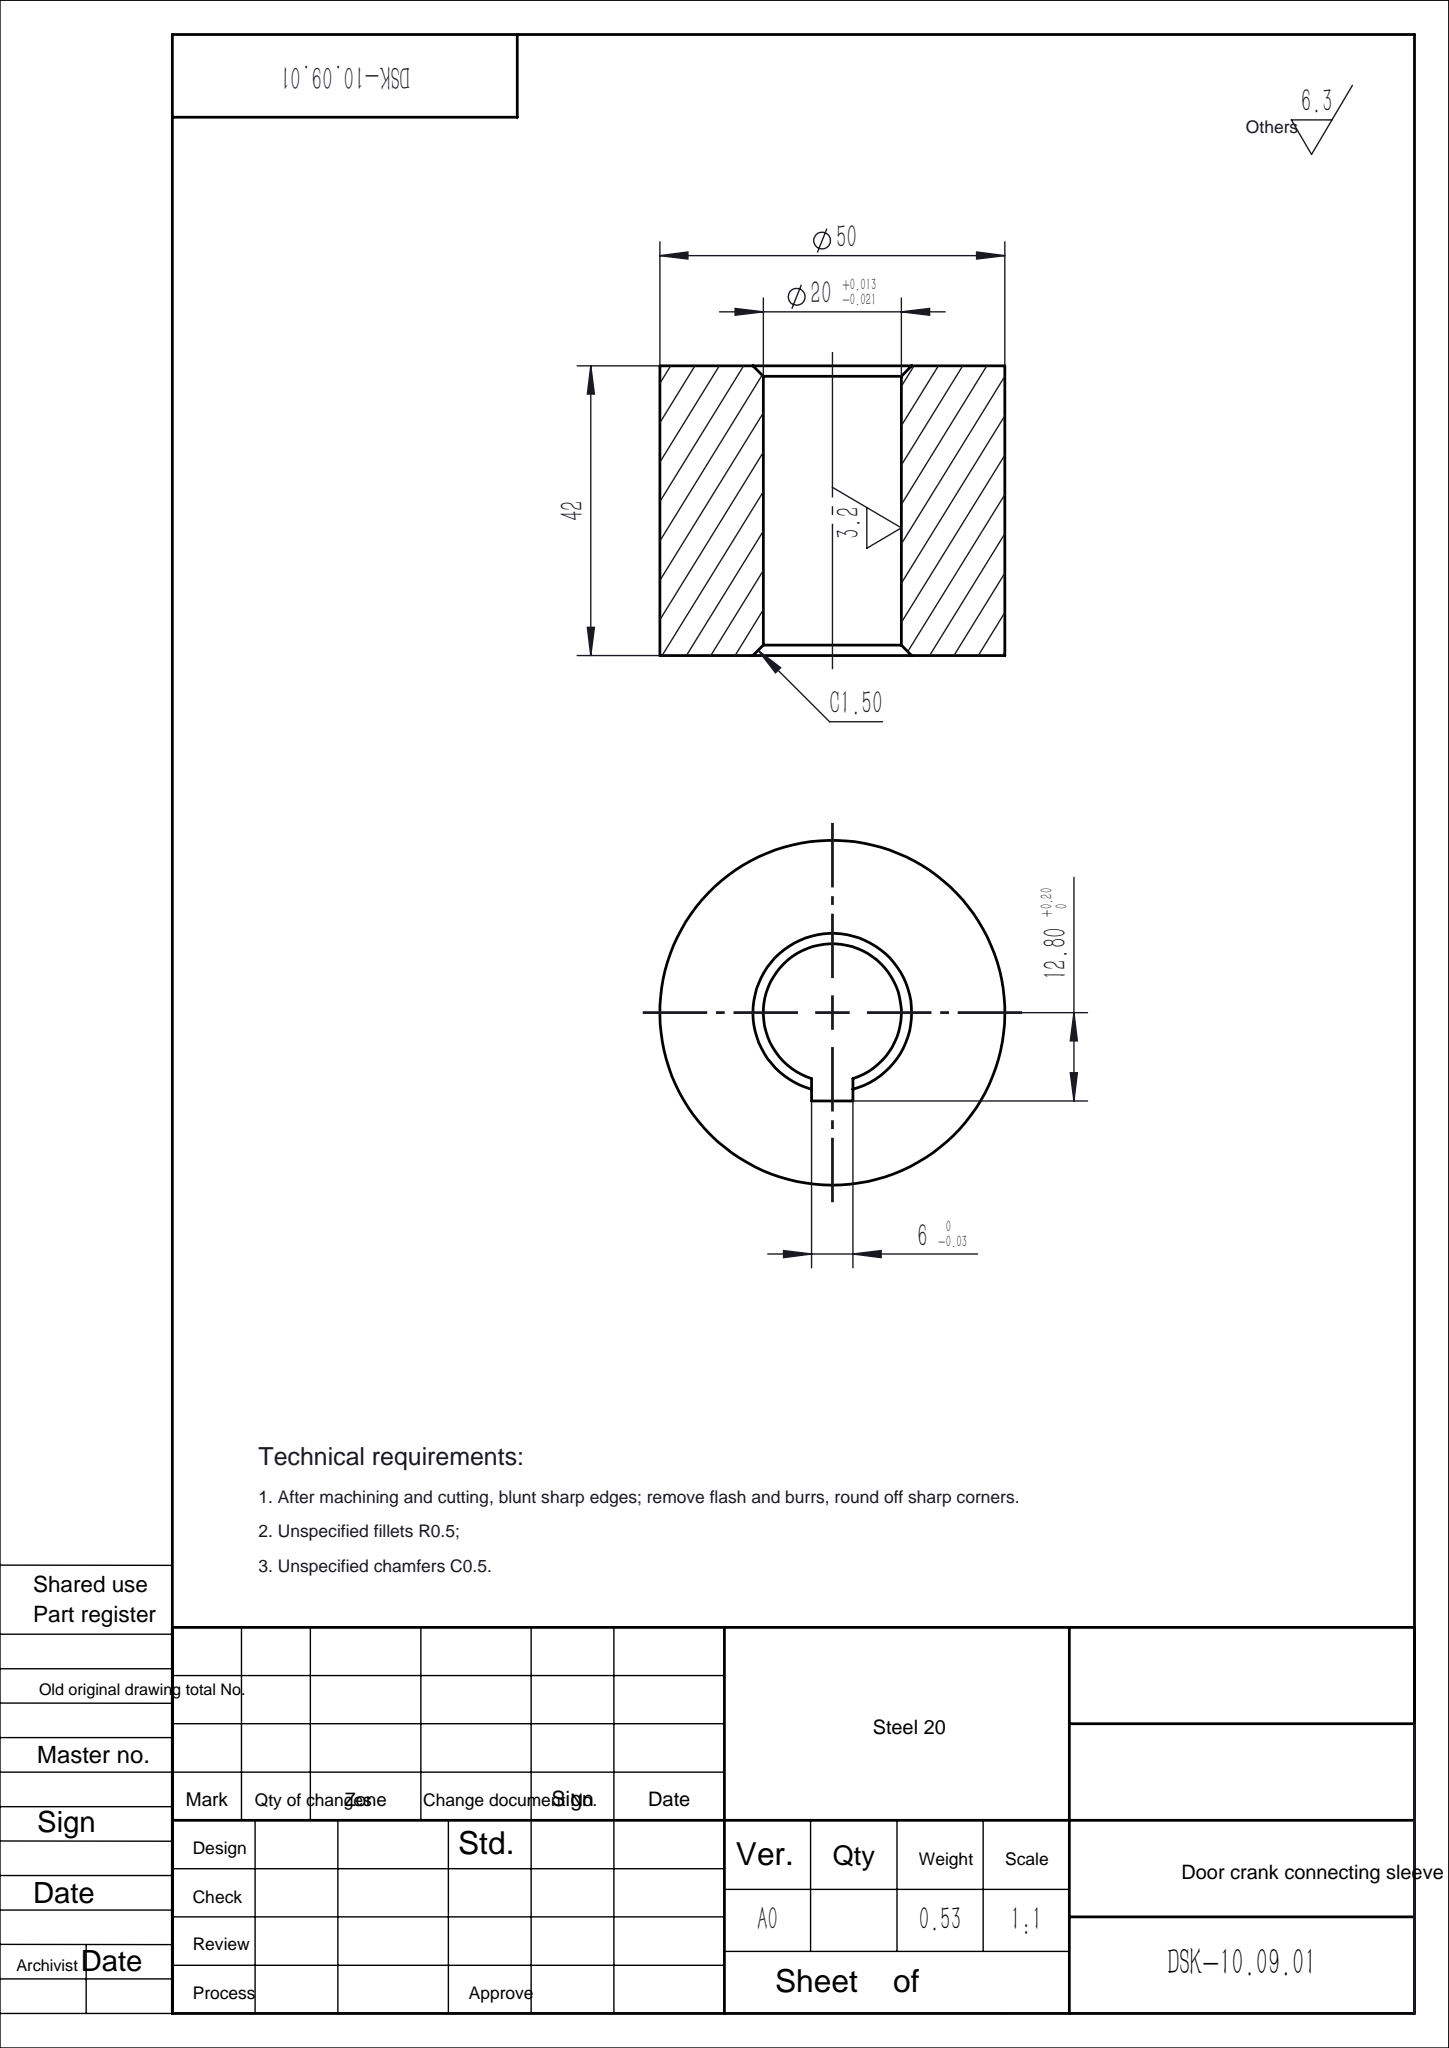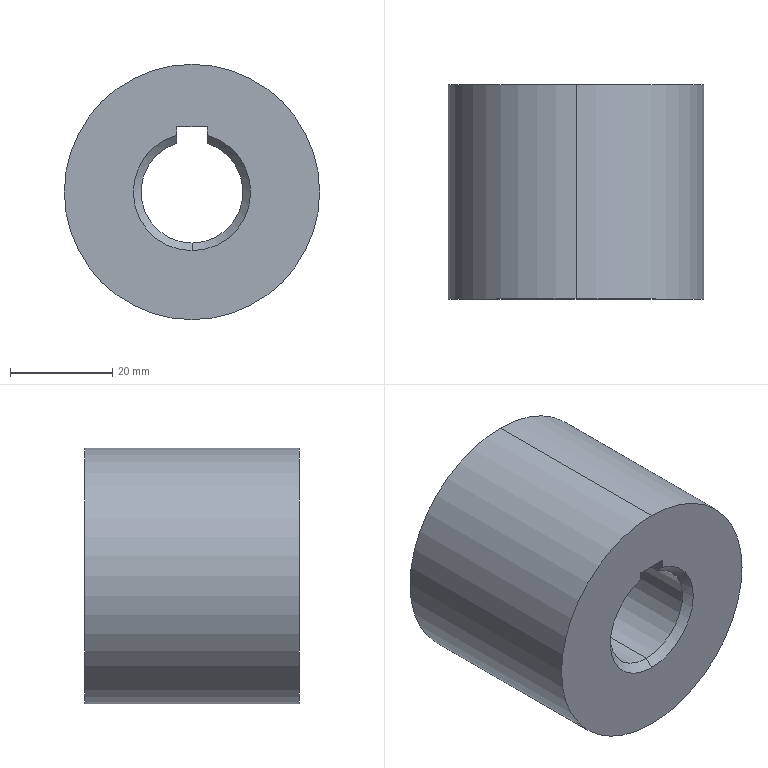Part | SolidWorks | features Chamfer 1, Extrusion 1 | 1 solid | 12 faces | box 50 x 42 x 50 mm | volume 68393 mm3 | plane 5 | cylinder 4 | cone 3 | commonest cylinder face diameters 20 x2 50 x2
STEP:
#1=CARTESIAN_POINT('',(0.,1.5,-10.));
#2=VERTEX_POINT('',#1);
#3=CARTESIAN_POINT('',(3.,1.5,9.539));
#4=VERTEX_POINT('',#3);
#5=CARTESIAN_POINT('',(0.,1.5,0.));
#6=DIRECTION('',(0.,-1.,0.));
#7=DIRECTION('',(0.,0.,1.));
#8=AXIS2_PLACEMENT_3D('',#5,#6,#7);
#9=CIRCLE('',#8,10.);
#10=EDGE_CURVE('',#2,#4,#9,.T.);
#11=ORIENTED_EDGE('',*,*,#10,.F.);
#12=CARTESIAN_POINT('',(0.,0.,-11.5));
#13=VERTEX_POINT('',#12);
#14=CARTESIAN_POINT('',(0.,0.,-11.5));
#15=DIRECTION('',(0.,-0.7071,-0.7071));
#16=VECTOR('',#15,1000.);
#17=LINE('',#14,#16);
#18=EDGE_CURVE('',#2,#13,#17,.T.);
#19=ORIENTED_EDGE('',*,*,#18,.T.);
#20=CARTESIAN_POINT('',(3.,0.,11.102));
#21=VERTEX_POINT('',#20);
#22=CARTESIAN_POINT('',(0.,0.,0.));
#23=DIRECTION('',(0.,1.,0.));
#24=DIRECTION('',(0.,0.,1.));
#25=AXIS2_PLACEMENT_3D('',#22,#23,#24);
#26=CIRCLE('',#25,11.5);
#27=EDGE_CURVE('',#21,#13,#26,.T.);
#28=ORIENTED_EDGE('',*,*,#27,.F.);
#29=CARTESIAN_POINT('',(3.,1.5,9.539));
#30=CARTESIAN_POINT('',(3.,1.002,10.062));
#31=CARTESIAN_POINT('',(3.,0.5014,10.582));
#32=CARTESIAN_POINT('',(3.,0.,11.102));
#33=B_SPLINE_CURVE_WITH_KNOTS('',3,(#29,#30,#31,#32),.UNSPECIFIED.,.F.,.F.,(4,4),(0.,0.002166),.UNSPECIFIED.);
#34=EDGE_CURVE('',#4,#21,#33,.T.);
#35=ORIENTED_EDGE('',*,*,#34,.F.);
#36=EDGE_LOOP('',(#11,#19,#28,#35));
#37=FACE_OUTER_BOUND('',#36,.T.);
#38=CARTESIAN_POINT('',(0.,0.,0.));
#39=DIRECTION('',(0.,-1.,0.));
#40=DIRECTION('',(0.,0.,-1.));
#41=AXIS2_PLACEMENT_3D('',#38,#39,#40);
#42=CONICAL_SURFACE('',#41,11.5,0.7854);
#43=ADVANCED_FACE('',(#37),#42,.F.);
#44=CARTESIAN_POINT('',(0.,42.,25.));
#45=VERTEX_POINT('',#44);
#46=CARTESIAN_POINT('',(0.,42.,-25.));
#47=VERTEX_POINT('',#46);
#48=CARTESIAN_POINT('',(0.,42.,0.));
#49=DIRECTION('',(0.,1.,0.));
#50=DIRECTION('',(0.,0.,1.));
#51=AXIS2_PLACEMENT_3D('',#48,#49,#50);
#52=CIRCLE('',#51,25.);
#53=EDGE_CURVE('',#45,#47,#52,.T.);
#54=ORIENTED_EDGE('',*,*,#53,.F.);
#55=CARTESIAN_POINT('',(0.,0.,25.));
#56=VERTEX_POINT('',#55);
#57=CARTESIAN_POINT('',(0.,42.,25.));
#58=DIRECTION('',(0.,-1.,0.));
#59=VECTOR('',#58,1000.);
#60=LINE('',#57,#59);
#61=EDGE_CURVE('',#45,#56,#60,.T.);
#62=ORIENTED_EDGE('',*,*,#61,.T.);
#63=CARTESIAN_POINT('',(0.,0.,-25.));
#64=VERTEX_POINT('',#63);
#65=CARTESIAN_POINT('',(0.,0.,0.));
#66=DIRECTION('',(0.,1.,0.));
#67=DIRECTION('',(0.,0.,1.));
#68=AXIS2_PLACEMENT_3D('',#65,#66,#67);
#69=CIRCLE('',#68,25.);
#70=EDGE_CURVE('',#56,#64,#69,.T.);
#71=ORIENTED_EDGE('',*,*,#70,.T.);
#72=CARTESIAN_POINT('',(0.,42.,-25.));
#73=DIRECTION('',(0.,-1.,0.));
#74=VECTOR('',#73,1000.);
#75=LINE('',#72,#74);
#76=EDGE_CURVE('',#47,#64,#75,.T.);
#77=ORIENTED_EDGE('',*,*,#76,.F.);
#78=EDGE_LOOP('',(#54,#62,#71,#77));
#79=FACE_OUTER_BOUND('',#78,.T.);
#80=CARTESIAN_POINT('',(0.,42.,0.));
#81=DIRECTION('',(0.,-1.,0.));
#82=DIRECTION('',(0.,0.,-1.));
#83=AXIS2_PLACEMENT_3D('',#80,#81,#82);
#84=CYLINDRICAL_SURFACE('',#83,25.);
#85=ADVANCED_FACE('',(#79),#84,.T.);
#86=CARTESIAN_POINT('',(3.,40.5,9.539));
#87=VERTEX_POINT('',#86);
#88=CARTESIAN_POINT('',(0.,40.5,-10.));
#89=VERTEX_POINT('',#88);
#90=CARTESIAN_POINT('',(0.,40.5,0.));
#91=DIRECTION('',(0.,1.,0.));
#92=DIRECTION('',(0.,0.,1.));
#93=AXIS2_PLACEMENT_3D('',#90,#91,#92);
#94=CIRCLE('',#93,10.);
#95=EDGE_CURVE('',#87,#89,#94,.T.);
#96=ORIENTED_EDGE('',*,*,#95,.T.);
#97=CARTESIAN_POINT('',(0.,42.,-10.));
#98=DIRECTION('',(0.,-1.,0.));
#99=VECTOR('',#98,1000.);
#100=LINE('',#97,#99);
#101=EDGE_CURVE('',#89,#2,#100,.T.);
#102=ORIENTED_EDGE('',*,*,#101,.T.);
#103=ORIENTED_EDGE('',*,*,#10,.T.);
#104=CARTESIAN_POINT('',(3.,42.,9.539));
#105=DIRECTION('',(0.,-1.,0.));
#106=VECTOR('',#105,1000.);
#107=LINE('',#104,#106);
#108=EDGE_CURVE('',#87,#4,#107,.T.);
#109=ORIENTED_EDGE('',*,*,#108,.F.);
#110=EDGE_LOOP('',(#96,#102,#103,#109));
#111=FACE_OUTER_BOUND('',#110,.T.);
#112=CARTESIAN_POINT('',(0.,42.,0.));
#113=DIRECTION('',(0.,-1.,0.));
#114=DIRECTION('',(0.,0.,-1.));
#115=AXIS2_PLACEMENT_3D('',#112,#113,#114);
#116=CYLINDRICAL_SURFACE('',#115,10.);
#117=ADVANCED_FACE('',(#111),#116,.F.);
#118=ORIENTED_EDGE('',*,*,#101,.F.);
#119=CARTESIAN_POINT('',(-3.,40.5,9.539));
#120=VERTEX_POINT('',#119);
#121=CARTESIAN_POINT('',(0.,40.5,0.));
#122=DIRECTION('',(0.,1.,0.));
#123=DIRECTION('',(0.,0.,1.));
#124=AXIS2_PLACEMENT_3D('',#121,#122,#123);
#125=CIRCLE('',#124,10.);
#126=EDGE_CURVE('',#89,#120,#125,.T.);
#127=ORIENTED_EDGE('',*,*,#126,.T.);
#128=CARTESIAN_POINT('',(-3.,1.5,9.539));
#129=VERTEX_POINT('',#128);
#130=CARTESIAN_POINT('',(-3.,42.,9.539));
#131=DIRECTION('',(0.,-1.,0.));
#132=VECTOR('',#131,1000.);
#133=LINE('',#130,#132);
#134=EDGE_CURVE('',#120,#129,#133,.T.);
#135=ORIENTED_EDGE('',*,*,#134,.T.);
#136=CARTESIAN_POINT('',(0.,1.5,0.));
#137=DIRECTION('',(0.,-1.,0.));
#138=DIRECTION('',(0.,0.,1.));
#139=AXIS2_PLACEMENT_3D('',#136,#137,#138);
#140=CIRCLE('',#139,10.);
#141=EDGE_CURVE('',#129,#2,#140,.T.);
#142=ORIENTED_EDGE('',*,*,#141,.T.);
#143=EDGE_LOOP('',(#118,#127,#135,#142));
#144=FACE_OUTER_BOUND('',#143,.T.);
#145=CARTESIAN_POINT('',(0.,42.,0.));
#146=DIRECTION('',(0.,-1.,0.));
#147=DIRECTION('',(0.,0.,-1.));
#148=AXIS2_PLACEMENT_3D('',#145,#146,#147);
#149=CYLINDRICAL_SURFACE('',#148,10.);
#150=ADVANCED_FACE('',(#144),#149,.F.);
#151=CARTESIAN_POINT('',(3.,42.,11.102));
#152=VERTEX_POINT('',#151);
#153=CARTESIAN_POINT('',(3.,42.,12.8));
#154=VERTEX_POINT('',#153);
#155=CARTESIAN_POINT('',(3.,42.,0.));
#156=DIRECTION('',(0.,0.,1.));
#157=VECTOR('',#156,1000.);
#158=LINE('',#155,#157);
#159=EDGE_CURVE('',#152,#154,#158,.T.);
#160=ORIENTED_EDGE('',*,*,#159,.F.);
#161=CARTESIAN_POINT('',(3.,42.,11.102));
#162=CARTESIAN_POINT('',(3.,41.499,10.582));
#163=CARTESIAN_POINT('',(3.,40.998,10.062));
#164=CARTESIAN_POINT('',(3.,40.5,9.539));
#165=B_SPLINE_CURVE_WITH_KNOTS('',3,(#161,#162,#163,#164),.UNSPECIFIED.,.F.,.F.,(4,4),(0.,0.002166),.UNSPECIFIED.);
#166=EDGE_CURVE('',#152,#87,#165,.T.);
#167=ORIENTED_EDGE('',*,*,#166,.T.);
#168=ORIENTED_EDGE('',*,*,#108,.T.);
#169=ORIENTED_EDGE('',*,*,#34,.T.);
#170=CARTESIAN_POINT('',(3.,0.,12.8));
#171=VERTEX_POINT('',#170);
#172=CARTESIAN_POINT('',(3.,0.,0.));
#173=DIRECTION('',(0.,0.,1.));
#174=VECTOR('',#173,1000.);
#175=LINE('',#172,#174);
#176=EDGE_CURVE('',#21,#171,#175,.T.);
#177=ORIENTED_EDGE('',*,*,#176,.T.);
#178=CARTESIAN_POINT('',(3.,42.,12.8));
#179=DIRECTION('',(0.,-1.,0.));
#180=VECTOR('',#179,1000.);
#181=LINE('',#178,#180);
#182=EDGE_CURVE('',#154,#171,#181,.T.);
#183=ORIENTED_EDGE('',*,*,#182,.F.);
#184=EDGE_LOOP('',(#160,#167,#168,#169,#177,#183));
#185=FACE_OUTER_BOUND('',#184,.T.);
#186=CARTESIAN_POINT('',(3.,42.,0.));
#187=DIRECTION('',(1.,0.,0.));
#188=DIRECTION('',(0.,0.,-1.));
#189=AXIS2_PLACEMENT_3D('',#186,#187,#188);
#190=PLANE('',#189);
#191=ADVANCED_FACE('',(#185),#190,.F.);
#192=CARTESIAN_POINT('',(-3.,0.,12.8));
#193=VERTEX_POINT('',#192);
#194=CARTESIAN_POINT('',(0.,0.,12.8));
#195=DIRECTION('',(-1.,0.,0.));
#196=VECTOR('',#195,1000.);
#197=LINE('',#194,#196);
#198=EDGE_CURVE('',#171,#193,#197,.T.);
#199=ORIENTED_EDGE('',*,*,#198,.T.);
#200=CARTESIAN_POINT('',(-3.,42.,12.8));
#201=VERTEX_POINT('',#200);
#202=CARTESIAN_POINT('',(-3.,42.,12.8));
#203=DIRECTION('',(0.,-1.,0.));
#204=VECTOR('',#203,1000.);
#205=LINE('',#202,#204);
#206=EDGE_CURVE('',#201,#193,#205,.T.);
#207=ORIENTED_EDGE('',*,*,#206,.F.);
#208=CARTESIAN_POINT('',(0.,42.,12.8));
#209=DIRECTION('',(-1.,0.,0.));
#210=VECTOR('',#209,1000.);
#211=LINE('',#208,#210);
#212=EDGE_CURVE('',#154,#201,#211,.T.);
#213=ORIENTED_EDGE('',*,*,#212,.F.);
#214=ORIENTED_EDGE('',*,*,#182,.T.);
#215=EDGE_LOOP('',(#199,#207,#213,#214));
#216=FACE_OUTER_BOUND('',#215,.T.);
#217=CARTESIAN_POINT('',(0.,42.,12.8));
#218=DIRECTION('',(0.,0.,1.));
#219=DIRECTION('',(1.,0.,0.));
#220=AXIS2_PLACEMENT_3D('',#217,#218,#219);
#221=PLANE('',#220);
#222=ADVANCED_FACE('',(#216),#221,.F.);
#223=ORIENTED_EDGE('',*,*,#134,.F.);
#224=CARTESIAN_POINT('',(-3.,42.,11.102));
#225=VERTEX_POINT('',#224);
#226=CARTESIAN_POINT('',(-3.,40.5,9.539));
#227=CARTESIAN_POINT('',(-3.,40.998,10.062));
#228=CARTESIAN_POINT('',(-3.,41.499,10.582));
#229=CARTESIAN_POINT('',(-3.,42.,11.102));
#230=B_SPLINE_CURVE_WITH_KNOTS('',3,(#226,#227,#228,#229),.UNSPECIFIED.,.F.,.F.,(4,4),(0.,0.002166),.UNSPECIFIED.);
#231=EDGE_CURVE('',#120,#225,#230,.T.);
#232=ORIENTED_EDGE('',*,*,#231,.T.);
#233=CARTESIAN_POINT('',(-3.,42.,0.));
#234=DIRECTION('',(0.,0.,1.));
#235=VECTOR('',#234,1000.);
#236=LINE('',#233,#235);
#237=EDGE_CURVE('',#225,#201,#236,.T.);
#238=ORIENTED_EDGE('',*,*,#237,.T.);
#239=ORIENTED_EDGE('',*,*,#206,.T.);
#240=CARTESIAN_POINT('',(-3.,0.,11.102));
#241=VERTEX_POINT('',#240);
#242=CARTESIAN_POINT('',(-3.,0.,0.));
#243=DIRECTION('',(0.,0.,1.));
#244=VECTOR('',#243,1000.);
#245=LINE('',#242,#244);
#246=EDGE_CURVE('',#241,#193,#245,.T.);
#247=ORIENTED_EDGE('',*,*,#246,.F.);
#248=CARTESIAN_POINT('',(-3.,0.,11.102));
#249=CARTESIAN_POINT('',(-3.,0.5014,10.582));
#250=CARTESIAN_POINT('',(-3.,1.002,10.062));
#251=CARTESIAN_POINT('',(-3.,1.5,9.539));
#252=B_SPLINE_CURVE_WITH_KNOTS('',3,(#248,#249,#250,#251),.UNSPECIFIED.,.F.,.F.,(4,4),(0.,0.002166),.UNSPECIFIED.);
#253=EDGE_CURVE('',#241,#129,#252,.T.);
#254=ORIENTED_EDGE('',*,*,#253,.T.);
#255=EDGE_LOOP('',(#223,#232,#238,#239,#247,#254));
#256=FACE_OUTER_BOUND('',#255,.T.);
#257=CARTESIAN_POINT('',(-3.,42.,0.));
#258=DIRECTION('',(1.,0.,0.));
#259=DIRECTION('',(0.,0.,-1.));
#260=AXIS2_PLACEMENT_3D('',#257,#258,#259);
#261=PLANE('',#260);
#262=ADVANCED_FACE('',(#256),#261,.T.);
#263=ORIENTED_EDGE('',*,*,#61,.F.);
#264=CARTESIAN_POINT('',(0.,42.,0.));
#265=DIRECTION('',(0.,1.,0.));
#266=DIRECTION('',(0.,0.,1.));
#267=AXIS2_PLACEMENT_3D('',#264,#265,#266);
#268=CIRCLE('',#267,25.);
#269=EDGE_CURVE('',#47,#45,#268,.T.);
#270=ORIENTED_EDGE('',*,*,#269,.F.);
#271=ORIENTED_EDGE('',*,*,#76,.T.);
#272=CARTESIAN_POINT('',(0.,0.,0.));
#273=DIRECTION('',(0.,1.,0.));
#274=DIRECTION('',(0.,0.,1.));
#275=AXIS2_PLACEMENT_3D('',#272,#273,#274);
#276=CIRCLE('',#275,25.);
#277=EDGE_CURVE('',#64,#56,#276,.T.);
#278=ORIENTED_EDGE('',*,*,#277,.T.);
#279=EDGE_LOOP('',(#263,#270,#271,#278));
#280=FACE_OUTER_BOUND('',#279,.T.);
#281=CARTESIAN_POINT('',(0.,42.,0.));
#282=DIRECTION('',(0.,-1.,0.));
#283=DIRECTION('',(0.,0.,-1.));
#284=AXIS2_PLACEMENT_3D('',#281,#282,#283);
#285=CYLINDRICAL_SURFACE('',#284,25.);
#286=ADVANCED_FACE('',(#280),#285,.T.);
#287=ORIENTED_EDGE('',*,*,#237,.F.);
#288=CARTESIAN_POINT('',(0.,42.,0.));
#289=DIRECTION('',(0.,-1.,0.));
#290=DIRECTION('',(0.,0.,1.));
#291=AXIS2_PLACEMENT_3D('',#288,#289,#290);
#292=CIRCLE('',#291,11.5);
#293=EDGE_CURVE('',#225,#152,#292,.T.);
#294=ORIENTED_EDGE('',*,*,#293,.T.);
#295=ORIENTED_EDGE('',*,*,#159,.T.);
#296=ORIENTED_EDGE('',*,*,#212,.T.);
#297=EDGE_LOOP('',(#287,#294,#295,#296));
#298=FACE_BOUND('',#297,.T.);
#299=ORIENTED_EDGE('',*,*,#269,.T.);
#300=ORIENTED_EDGE('',*,*,#53,.T.);
#301=EDGE_LOOP('',(#299,#300));
#302=FACE_OUTER_BOUND('',#301,.T.);
#303=CARTESIAN_POINT('',(0.,42.,0.));
#304=DIRECTION('',(0.,1.,0.));
#305=DIRECTION('',(0.,0.,1.));
#306=AXIS2_PLACEMENT_3D('',#303,#304,#305);
#307=PLANE('',#306);
#308=ADVANCED_FACE('',(#298,#302),#307,.T.);
#309=ORIENTED_EDGE('',*,*,#176,.F.);
#310=ORIENTED_EDGE('',*,*,#27,.T.);
#311=CARTESIAN_POINT('',(0.,0.,0.));
#312=DIRECTION('',(0.,1.,0.));
#313=DIRECTION('',(0.,0.,1.));
#314=AXIS2_PLACEMENT_3D('',#311,#312,#313);
#315=CIRCLE('',#314,11.5);
#316=EDGE_CURVE('',#13,#241,#315,.T.);
#317=ORIENTED_EDGE('',*,*,#316,.T.);
#318=ORIENTED_EDGE('',*,*,#246,.T.);
#319=ORIENTED_EDGE('',*,*,#198,.F.);
#320=EDGE_LOOP('',(#309,#310,#317,#318,#319));
#321=FACE_BOUND('',#320,.T.);
#322=ORIENTED_EDGE('',*,*,#277,.F.);
#323=ORIENTED_EDGE('',*,*,#70,.F.);
#324=EDGE_LOOP('',(#322,#323));
#325=FACE_OUTER_BOUND('',#324,.T.);
#326=CARTESIAN_POINT('',(0.,0.,0.));
#327=DIRECTION('',(0.,1.,0.));
#328=DIRECTION('',(0.,0.,1.));
#329=AXIS2_PLACEMENT_3D('',#326,#327,#328);
#330=PLANE('',#329);
#331=ADVANCED_FACE('',(#321,#325),#330,.F.);
#332=ORIENTED_EDGE('',*,*,#166,.F.);
#333=ORIENTED_EDGE('',*,*,#293,.F.);
#334=ORIENTED_EDGE('',*,*,#231,.F.);
#335=ORIENTED_EDGE('',*,*,#126,.F.);
#336=ORIENTED_EDGE('',*,*,#95,.F.);
#337=EDGE_LOOP('',(#332,#333,#334,#335,#336));
#338=FACE_OUTER_BOUND('',#337,.T.);
#339=CARTESIAN_POINT('',(0.,40.5,0.));
#340=DIRECTION('',(0.,1.,0.));
#341=DIRECTION('',(0.,0.,1.));
#342=AXIS2_PLACEMENT_3D('',#339,#340,#341);
#343=CONICAL_SURFACE('',#342,10.,0.7854);
#344=ADVANCED_FACE('',(#338),#343,.F.);
#345=ORIENTED_EDGE('',*,*,#18,.F.);
#346=ORIENTED_EDGE('',*,*,#141,.F.);
#347=ORIENTED_EDGE('',*,*,#253,.F.);
#348=ORIENTED_EDGE('',*,*,#316,.F.);
#349=EDGE_LOOP('',(#345,#346,#347,#348));
#350=FACE_OUTER_BOUND('',#349,.T.);
#351=CARTESIAN_POINT('',(0.,0.,0.));
#352=DIRECTION('',(0.,-1.,0.));
#353=DIRECTION('',(0.,0.,-1.));
#354=AXIS2_PLACEMENT_3D('',#351,#352,#353);
#355=CONICAL_SURFACE('',#354,11.5,0.7854);
#356=ADVANCED_FACE('',(#350),#355,.F.);
#357=CLOSED_SHELL('',(#43,#85,#117,#150,#191,#222,#262,#286,#308,#331,#344,#356));
#358=MANIFOLD_SOLID_BREP('',#357);
#359=CARTESIAN_POINT('',(0.,0.,0.));
#360=DIRECTION('',(0.,0.,1.));
#361=DIRECTION('',(1.,0.,0.));
#362=AXIS2_PLACEMENT_3D('',#359,#360,#361);
#363=(LENGTH_UNIT()NAMED_UNIT(*)SI_UNIT(.MILLI.,.METRE.));
#364=UNCERTAINTY_MEASURE_WITH_UNIT(LENGTH_MEASURE(0.00001),#363,'','');
#365=(NAMED_UNIT(*)PLANE_ANGLE_UNIT()SI_UNIT($,.RADIAN.));
#366=(NAMED_UNIT(*)SI_UNIT($,.STERADIAN.)SOLID_ANGLE_UNIT());
#367=(GEOMETRIC_REPRESENTATION_CONTEXT(3)GLOBAL_UNCERTAINTY_ASSIGNED_CONTEXT((#364))GLOBAL_UNIT_ASSIGNED_CONTEXT((#363,#365,#366))REPRESENTATION_CONTEXT('',''));
#368=ADVANCED_BREP_SHAPE_REPRESENTATION('',(#358,#362),#367);